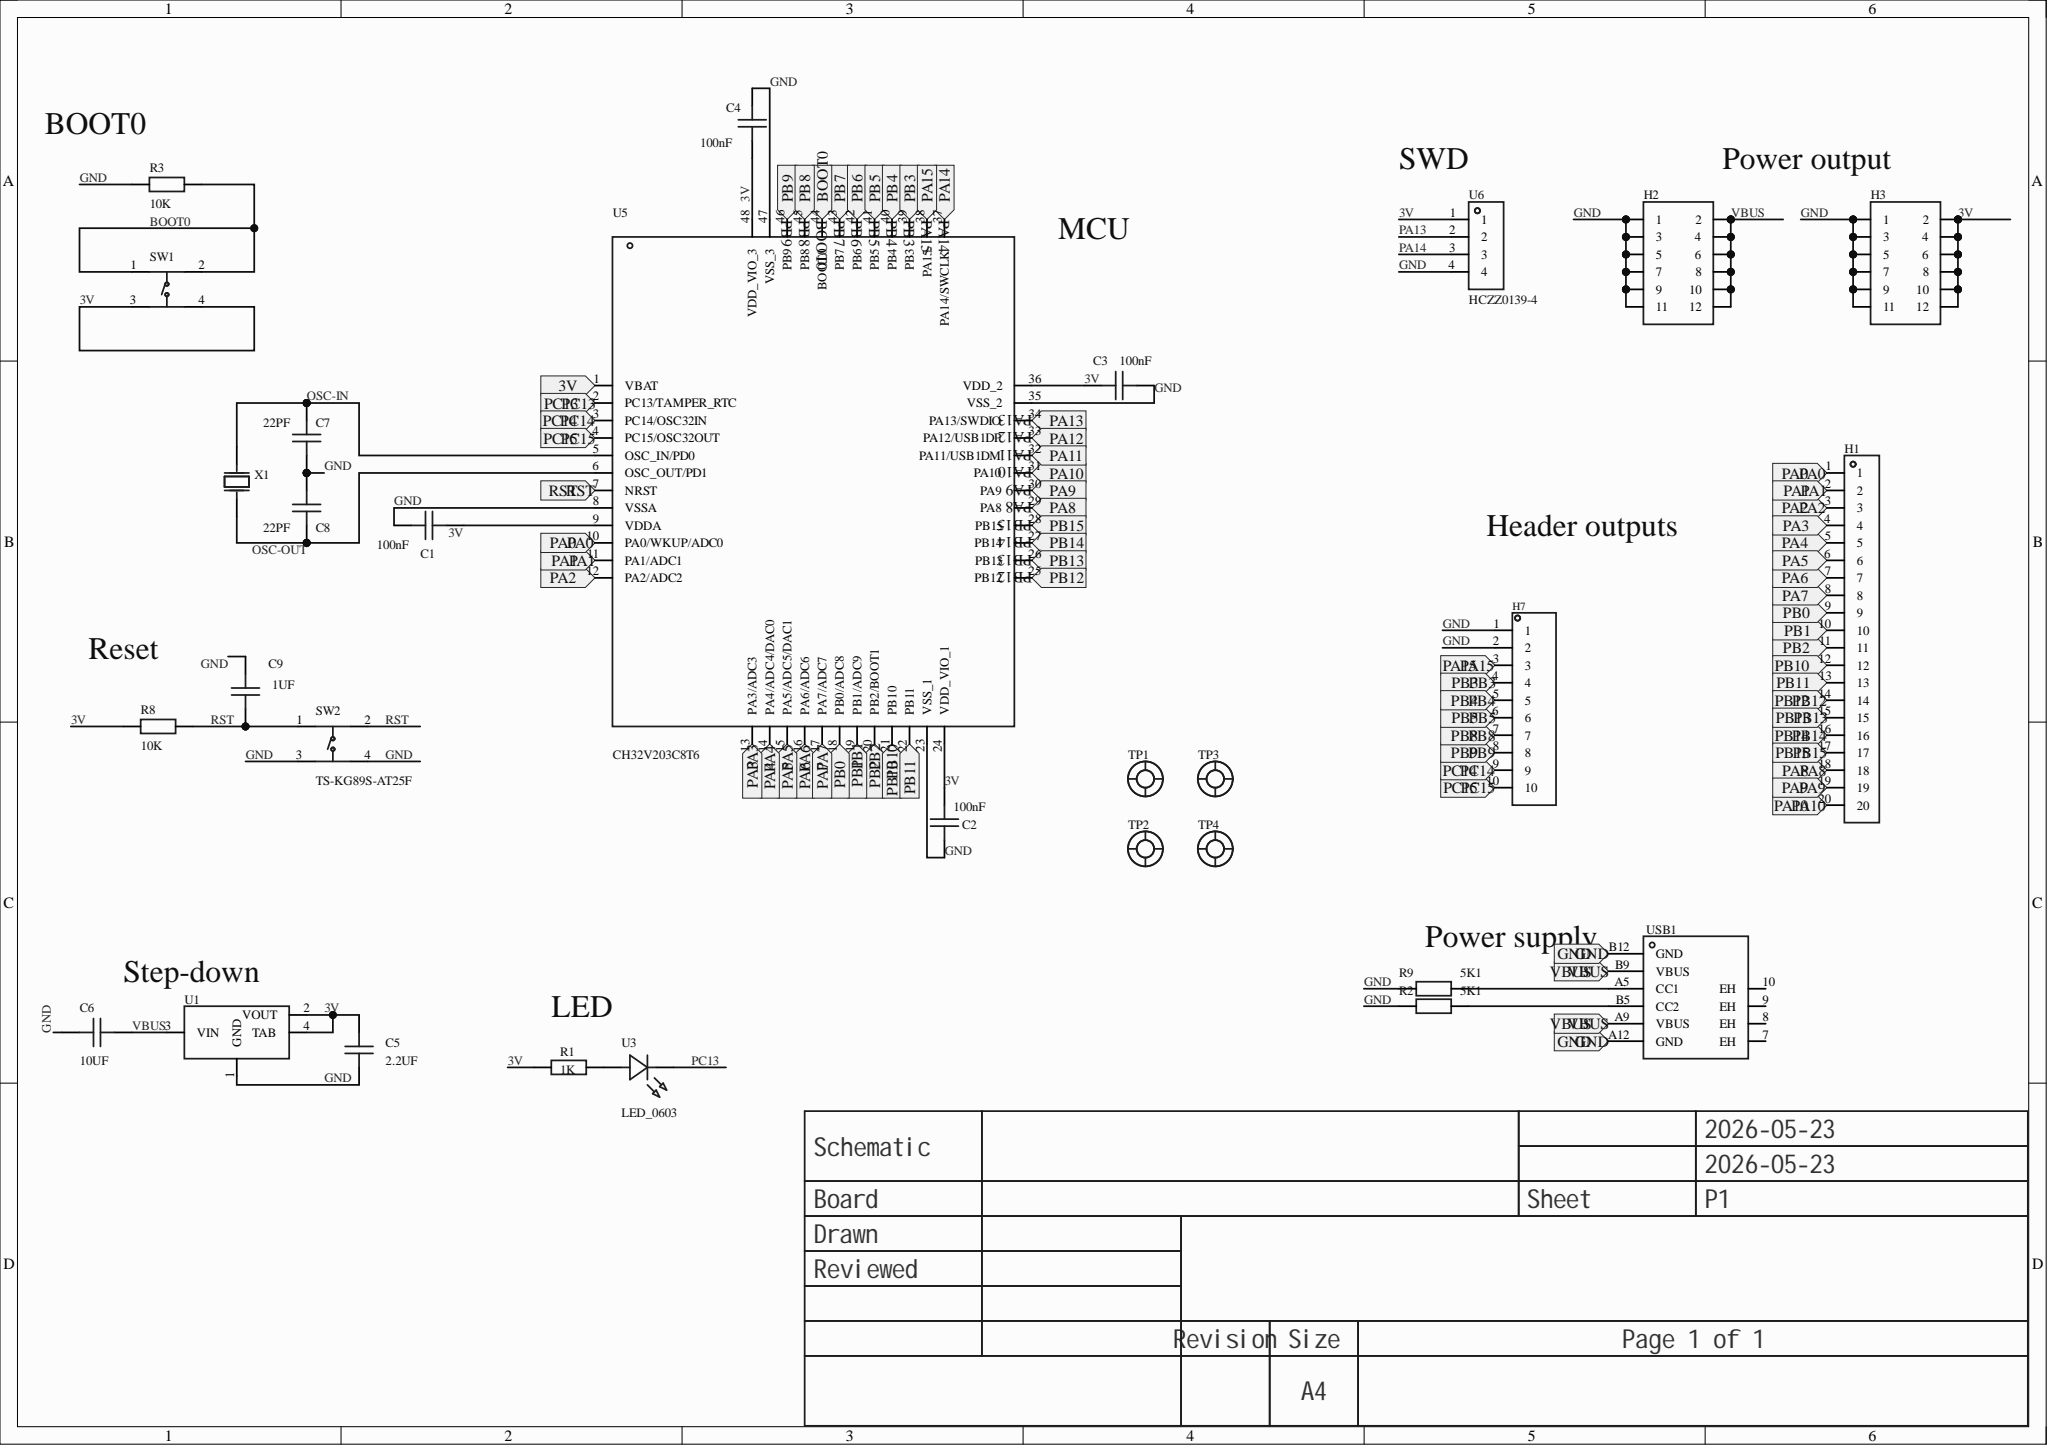Circuit board | Altium Designer | 30 parts | 41 nets
Bill of materials:
Comment,Description,Designator,Footprint,LibRef,Quantity
"100nF","","C1, C2, C3, C4","C0603","CAP_0603","4"
"2.2UF","","C5","C0603","CAP_0603","1"
"10UF","","C6","C0603","CAP_0603","1"
"22PF","","C7, C8","C0603","CAP_0603","2"
"1UF","","C9","C0603","CAP_0603","1"
"","Pitch:2.54mm;Total pins:20;Rows:1;Pin structure:-;Row spacing:-;Mounting type:Through-hole;Round/square pin:-;Rated current:-;Rated voltage:-;Mating pin length:-;Plastic height:-;Contact material:Brass;Contact plating:-;Color:Black;","H1","HDR-TH_20P-P2.54-V-M-1","HDR-M_2.54_1x20P","1"
"","","H2, H3","HDR-TH_12P-P2.54-V-M-R2-C6-S2.54","HDR-F_2.54_2x6","2"
"","","H7","hdr-th_10p-p2.54-v-m-1","HDR-M_2.54_1x10P","1"
"1K","","R1","R0603","Res_0603","1"
"5K1","","R2, R9","R0603","Res_0603","2"
"10K","","R3, R8","R0603","Res_0603","2"
"TS-KG89S-AT25F","","SW1, SW2","SW-SMD_4P-L4.2-W3.3-P2.15-LS5.1","4.2*3.25*2.5mm-立贴-轻触开关","2"
"","","TP1, TP2, TP3, TP4","M3","M3","4"
"","","U1","SOT_223","AMS1117","1"
"LED_0603","","U3","LED_0603","LED_0603_W","1"
"CH32V203C8T6","CPU core:RISC-V;Program storage capacity:64KB;Total RAM:20KB;GPIO port count:-;Operating voltage range:-;Max CPU frequency:144MHz;Program memory type:FLASH;","U5","LQFP-48_L7.0-W7.0-P0.50-LS9.0-BL","CH32V203C8T6","1"
"HCZZ0139-4","Pin structure:1x4P;Pitch:2.54mm;Mounting:Right-angle THT;Reference series:XH;Total pins:4P;Rows:1;Pins per row:4;Rated current:3A;Contact material:Brass;Contact plating:Tin;Operating temperature range:-25℃~+85℃;","U6","CONN-TH_4P-P2.50_HCZZ0139-4","XH2.54_弯针_x4P","1"
"","","USB1","USB_ TYPE-C-6P","USB_ Type-C-6P","1"
"8M-HC-49SMD","","X1","CRYSTAL-SMD_L11.4-W4.7-LS12.7","HC-49SMD","1"
Netlist (Protel format):
[
C1
C0603
100nF



]
[
C2
C0603
100nF



]
[
C3
C0603
100nF



]
[
C4
C0603
100nF



]
[
C5
C0603
2.2UF



]
[
C6
C0603
10UF



]
[
C7
C0603
22PF



]
[
C8
C0603
22PF



]
[
C9
C0603
1UF



]
[
H1
HDR-TH_20P-P2.54-V-M-1




]
[
H2
HDR-TH_12P-P2.54-V-M-R2-C6-S2.54




]
[
H3
HDR-TH_12P-P2.54-V-M-R2-C6-S2.54




]
[
H7
hdr-th_10p-p2.54-v-m-1




]
[
R1
R0603
1K



]
[
R2
R0603
5K1



]
[
R3
R0603
10K



]
[
R8
R0603
10K



]
[
R9
R0603
5K1



]
[
SW1
SW-SMD_4P-L4.2-W3.3-P2.15-LS5.1
TS-KG89S-AT25F



]
[
SW2
SW-SMD_4P-L4.2-W3.3-P2.15-LS5.1
TS-KG89S-AT25F



]
[
TP1
M3




]
[
TP2
M3




]
[
TP3
M3




]
[
TP4
M3




]
[
U1
SOT_223




]
[
U3
LED_0603
LED_0603



]
[
U5
LQFP-48_L7.0-W7.0-P0.50-LS9.0-BL
CH32V203C8T6



]
[
U6
CONN-TH_4P-P2.50_HCZZ0139-4
HCZZ0139-4



]
[
USB1
USB_ TYPE-C-6P




]
[
X1
CRYSTAL-SMD_L11.4-W4.7-LS12.7
8M-HC-49SMD



]
(
VBUS
C6-2
H2-2
H2-4
H2-6
H2-8
H2-10
H2-12
U1-3
USB1-A9
USB1-B9
)
(
RST
C9-1
R8-2
SW2-1
SW2-2
U5-7
)
(
PC15
H7-10
U5-4
)
(
PC14
H7-9
U5-3
)
(
PC13
U3-1
U5-2
)
(
PB15
H1-17
U5-28
)
(
PB14
H1-16
U5-27
)
(
PB13
H1-15
U5-26
)
(
PB12
H1-14
U5-25
)
(
PB10
H1-12
U5-21
)
(
PB9
H7-8
U5-46
)
(
PB8
H7-7
U5-45
)
(
PB5
H7-6
U5-41
)
(
PB4
H7-5
U5-40
)
(
PB3
H7-4
U5-39
)
(
PB2
H1-11
U5-20
)
(
PB1
H1-10
U5-19
)
(
PA15
H7-3
U5-38
)
(
PA14
U5-37
U6-3
)
(
PA13
U5-34
U6-2
)
(
PA10
H1-20
U5-31
)
(
PA9
H1-19
U5-30
)
(
PA8
H1-18
U5-29
)
(
PA7
H1-8
U5-17
)
(
PA6
H1-7
U5-16
)
(
PA5
H1-6
U5-15
)
(
PA4
H1-5
U5-14
)
(
PA3
H1-4
U5-13
)
(
PA2
H1-3
U5-12
)
(
PA1
H1-2
U5-11
)
(
PA0
H1-1
U5-10
)
(
OSC-OUT
C8-1
U5-6
X1-1
)
(
OSC-IN
C7-2
U5-5
X1-2
)
(
NetR9_2
R9-2
USB1-A5
)
(
NetR2_2
R2-2
USB1-B5
)
(
NetR1_2
R1-2
U3-2
)
(
NetH1_13
H1-13
U5-22
)
(
NetH1_9
H1-9
U5-18
)
(
GND
C1-2
C2-1
C3-1
C4-2
C5-2
C6-1
C7-1
C8-2
C9-2
H2-1
H2-3
H2-5
H2-7
H2-9
H2-11
H3-1
H3-3
H3-5
H3-7
H3-9
H3-11
H7-1
H7-2
R2-1
R3-1
R9-1
SW2-3
SW2-4
U1-1
U5-8
U5-23
U5-35
U5-47
U6-4
USB1-A12
USB1-B12
)
(
BOOT0
R3-2
SW1-1
SW1-2
U5-44
)
(
3V
C1-1
C2-2
C3-2
C4-1
C5-1
H3-2
H3-4
H3-6
H3-8
H3-10
H3-12
R1-1
R8-1
SW1-3
SW1-4
U1-2
U1-4
U5-9
U5-24
U5-36
U5-48
U6-1
)